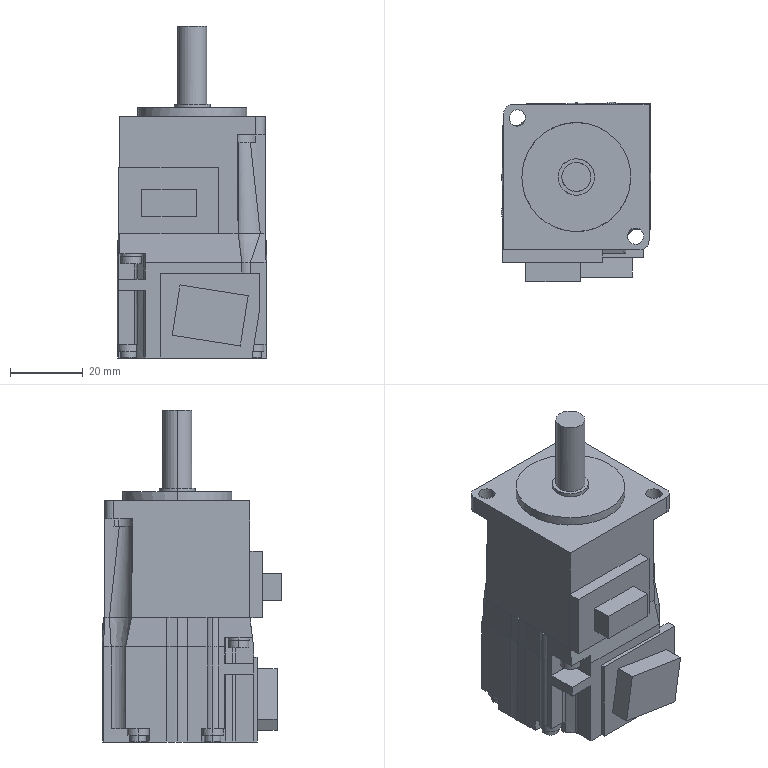Part | STEP file | PN_0007hg-kr053_ | 1 solid | 186 faces | box 41.201 x 49.5 x 91.4 mm | volume 107634 mm3 | plane 106 | cylinder 68 | spline 9 | cone 3 | commonest cylinder face diameters 4.5 x12 2 x8 6 x8 8 x5 5.6 x4 5.9 x4